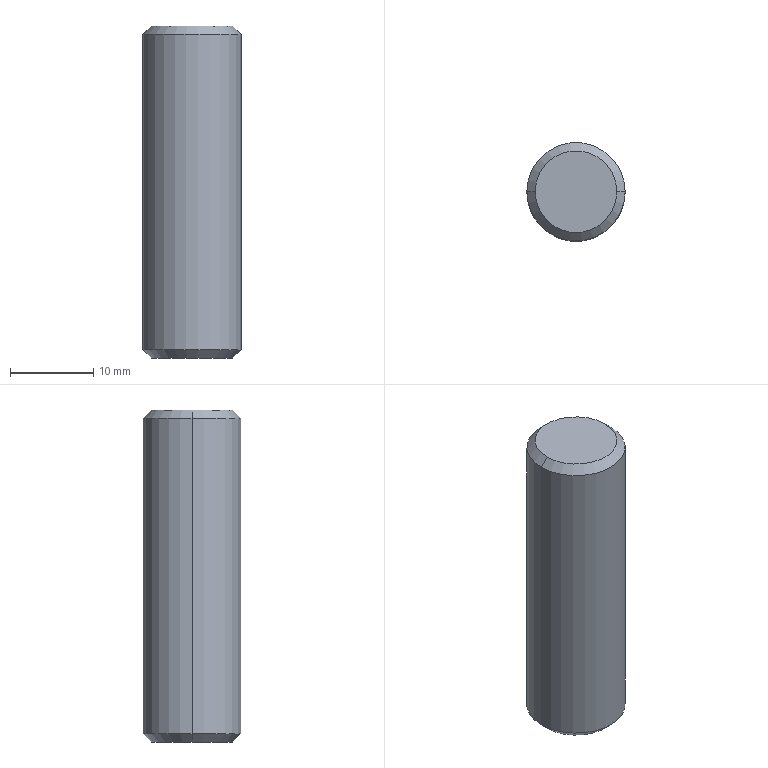Part | SolidWorks | features Chamfer 1, Extrusion 1 | 1 solid | 8 faces | box 11.85 x 11.85 x 40 mm | volume 4376 mm3 | cone 4 | cylinder 2 | plane 2 | commonest cylinder face diameters 11.85 x2
STEP:
#1=CARTESIAN_POINT('',(-4.925,0.,0.));
#2=VERTEX_POINT('',#1);
#3=CARTESIAN_POINT('',(4.925,0.,0.));
#4=VERTEX_POINT('',#3);
#5=CARTESIAN_POINT('',(0.,0.,0.));
#6=DIRECTION('',(0.,0.,-1.));
#7=DIRECTION('',(1.,0.,0.));
#8=AXIS2_PLACEMENT_3D('',#5,#6,#7);
#9=CIRCLE('',#8,4.925);
#10=EDGE_CURVE('',#2,#4,#9,.T.);
#11=ORIENTED_EDGE('',*,*,#10,.F.);
#12=CARTESIAN_POINT('',(-5.925,0.,1.));
#13=VERTEX_POINT('',#12);
#14=CARTESIAN_POINT('',(-5.925,0.,1.));
#15=DIRECTION('',(-0.7071,0.,0.7071));
#16=VECTOR('',#15,1000.);
#17=LINE('',#14,#16);
#18=EDGE_CURVE('',#2,#13,#17,.T.);
#19=ORIENTED_EDGE('',*,*,#18,.T.);
#20=CARTESIAN_POINT('',(5.925,0.,1.));
#21=VERTEX_POINT('',#20);
#22=CARTESIAN_POINT('',(0.,0.,1.));
#23=DIRECTION('',(0.,0.,1.));
#24=DIRECTION('',(1.,0.,0.));
#25=AXIS2_PLACEMENT_3D('',#22,#23,#24);
#26=CIRCLE('',#25,5.925);
#27=EDGE_CURVE('',#21,#13,#26,.T.);
#28=ORIENTED_EDGE('',*,*,#27,.F.);
#29=CARTESIAN_POINT('',(5.925,0.,1.));
#30=DIRECTION('',(0.7071,0.,0.7071));
#31=VECTOR('',#30,1000.);
#32=LINE('',#29,#31);
#33=EDGE_CURVE('',#4,#21,#32,.T.);
#34=ORIENTED_EDGE('',*,*,#33,.F.);
#35=EDGE_LOOP('',(#11,#19,#28,#34));
#36=FACE_OUTER_BOUND('',#35,.T.);
#37=CARTESIAN_POINT('',(0.,0.,1.));
#38=DIRECTION('',(0.,0.,1.));
#39=DIRECTION('',(1.,0.,0.));
#40=AXIS2_PLACEMENT_3D('',#37,#38,#39);
#41=CONICAL_SURFACE('',#40,5.925,0.7854);
#42=ADVANCED_FACE('',(#36),#41,.T.);
#43=CARTESIAN_POINT('',(4.925,0.,40.));
#44=VERTEX_POINT('',#43);
#45=CARTESIAN_POINT('',(-4.925,0.,40.));
#46=VERTEX_POINT('',#45);
#47=CARTESIAN_POINT('',(0.,0.,40.));
#48=DIRECTION('',(0.,0.,1.));
#49=DIRECTION('',(1.,0.,0.));
#50=AXIS2_PLACEMENT_3D('',#47,#48,#49);
#51=CIRCLE('',#50,4.925);
#52=EDGE_CURVE('',#44,#46,#51,.T.);
#53=ORIENTED_EDGE('',*,*,#52,.F.);
#54=CARTESIAN_POINT('',(5.925,0.,39.));
#55=VERTEX_POINT('',#54);
#56=CARTESIAN_POINT('',(4.925,0.,40.));
#57=DIRECTION('',(0.7071,0.,-0.7071));
#58=VECTOR('',#57,1000.);
#59=LINE('',#56,#58);
#60=EDGE_CURVE('',#44,#55,#59,.T.);
#61=ORIENTED_EDGE('',*,*,#60,.T.);
#62=CARTESIAN_POINT('',(-5.925,0.,39.));
#63=VERTEX_POINT('',#62);
#64=CARTESIAN_POINT('',(0.,0.,39.));
#65=DIRECTION('',(0.,0.,-1.));
#66=DIRECTION('',(1.,0.,0.));
#67=AXIS2_PLACEMENT_3D('',#64,#65,#66);
#68=CIRCLE('',#67,5.925);
#69=EDGE_CURVE('',#63,#55,#68,.T.);
#70=ORIENTED_EDGE('',*,*,#69,.F.);
#71=CARTESIAN_POINT('',(-4.925,0.,40.));
#72=DIRECTION('',(-0.7071,0.,-0.7071));
#73=VECTOR('',#72,1000.);
#74=LINE('',#71,#73);
#75=EDGE_CURVE('',#46,#63,#74,.T.);
#76=ORIENTED_EDGE('',*,*,#75,.F.);
#77=EDGE_LOOP('',(#53,#61,#70,#76));
#78=FACE_OUTER_BOUND('',#77,.T.);
#79=CARTESIAN_POINT('',(0.,0.,40.));
#80=DIRECTION('',(0.,0.,-1.));
#81=DIRECTION('',(-1.,0.,0.));
#82=AXIS2_PLACEMENT_3D('',#79,#80,#81);
#83=CONICAL_SURFACE('',#82,4.925,0.7854);
#84=ADVANCED_FACE('',(#78),#83,.T.);
#85=ORIENTED_EDGE('',*,*,#69,.T.);
#86=CARTESIAN_POINT('',(5.925,0.,40.));
#87=DIRECTION('',(0.,0.,-1.));
#88=VECTOR('',#87,1000.);
#89=LINE('',#86,#88);
#90=EDGE_CURVE('',#55,#21,#89,.T.);
#91=ORIENTED_EDGE('',*,*,#90,.T.);
#92=ORIENTED_EDGE('',*,*,#27,.T.);
#93=CARTESIAN_POINT('',(-5.925,0.,40.));
#94=DIRECTION('',(0.,0.,-1.));
#95=VECTOR('',#94,1000.);
#96=LINE('',#93,#95);
#97=EDGE_CURVE('',#63,#13,#96,.T.);
#98=ORIENTED_EDGE('',*,*,#97,.F.);
#99=EDGE_LOOP('',(#85,#91,#92,#98));
#100=FACE_OUTER_BOUND('',#99,.T.);
#101=CARTESIAN_POINT('',(0.,0.,40.));
#102=DIRECTION('',(0.,0.,-1.));
#103=DIRECTION('',(-1.,0.,0.));
#104=AXIS2_PLACEMENT_3D('',#101,#102,#103);
#105=CYLINDRICAL_SURFACE('',#104,5.925);
#106=ADVANCED_FACE('',(#100),#105,.T.);
#107=ORIENTED_EDGE('',*,*,#90,.F.);
#108=CARTESIAN_POINT('',(0.,0.,39.));
#109=DIRECTION('',(0.,0.,-1.));
#110=DIRECTION('',(1.,0.,0.));
#111=AXIS2_PLACEMENT_3D('',#108,#109,#110);
#112=CIRCLE('',#111,5.925);
#113=EDGE_CURVE('',#55,#63,#112,.T.);
#114=ORIENTED_EDGE('',*,*,#113,.T.);
#115=ORIENTED_EDGE('',*,*,#97,.T.);
#116=CARTESIAN_POINT('',(0.,0.,1.));
#117=DIRECTION('',(0.,0.,1.));
#118=DIRECTION('',(1.,0.,0.));
#119=AXIS2_PLACEMENT_3D('',#116,#117,#118);
#120=CIRCLE('',#119,5.925);
#121=EDGE_CURVE('',#13,#21,#120,.T.);
#122=ORIENTED_EDGE('',*,*,#121,.T.);
#123=EDGE_LOOP('',(#107,#114,#115,#122));
#124=FACE_OUTER_BOUND('',#123,.T.);
#125=CARTESIAN_POINT('',(0.,0.,40.));
#126=DIRECTION('',(0.,0.,-1.));
#127=DIRECTION('',(-1.,0.,0.));
#128=AXIS2_PLACEMENT_3D('',#125,#126,#127);
#129=CYLINDRICAL_SURFACE('',#128,5.925);
#130=ADVANCED_FACE('',(#124),#129,.T.);
#131=CARTESIAN_POINT('',(0.,0.,40.));
#132=DIRECTION('',(0.,0.,1.));
#133=DIRECTION('',(1.,0.,0.));
#134=AXIS2_PLACEMENT_3D('',#131,#132,#133);
#135=CIRCLE('',#134,4.925);
#136=EDGE_CURVE('',#46,#44,#135,.T.);
#137=ORIENTED_EDGE('',*,*,#136,.T.);
#138=ORIENTED_EDGE('',*,*,#52,.T.);
#139=EDGE_LOOP('',(#137,#138));
#140=FACE_OUTER_BOUND('',#139,.T.);
#141=CARTESIAN_POINT('',(0.,0.,40.));
#142=DIRECTION('',(0.,0.,1.));
#143=DIRECTION('',(1.,0.,0.));
#144=AXIS2_PLACEMENT_3D('',#141,#142,#143);
#145=PLANE('',#144);
#146=ADVANCED_FACE('',(#140),#145,.T.);
#147=CARTESIAN_POINT('',(0.,0.,0.));
#148=DIRECTION('',(0.,0.,-1.));
#149=DIRECTION('',(1.,0.,0.));
#150=AXIS2_PLACEMENT_3D('',#147,#148,#149);
#151=CIRCLE('',#150,4.925);
#152=EDGE_CURVE('',#4,#2,#151,.T.);
#153=ORIENTED_EDGE('',*,*,#152,.T.);
#154=ORIENTED_EDGE('',*,*,#10,.T.);
#155=EDGE_LOOP('',(#153,#154));
#156=FACE_OUTER_BOUND('',#155,.T.);
#157=CARTESIAN_POINT('',(0.,0.,0.));
#158=DIRECTION('',(0.,0.,1.));
#159=DIRECTION('',(1.,0.,0.));
#160=AXIS2_PLACEMENT_3D('',#157,#158,#159);
#161=PLANE('',#160);
#162=ADVANCED_FACE('',(#156),#161,.F.);
#163=ORIENTED_EDGE('',*,*,#60,.F.);
#164=ORIENTED_EDGE('',*,*,#136,.F.);
#165=ORIENTED_EDGE('',*,*,#75,.T.);
#166=ORIENTED_EDGE('',*,*,#113,.F.);
#167=EDGE_LOOP('',(#163,#164,#165,#166));
#168=FACE_OUTER_BOUND('',#167,.T.);
#169=CARTESIAN_POINT('',(0.,0.,40.));
#170=DIRECTION('',(0.,0.,-1.));
#171=DIRECTION('',(-1.,0.,0.));
#172=AXIS2_PLACEMENT_3D('',#169,#170,#171);
#173=CONICAL_SURFACE('',#172,4.925,0.7854);
#174=ADVANCED_FACE('',(#168),#173,.T.);
#175=ORIENTED_EDGE('',*,*,#18,.F.);
#176=ORIENTED_EDGE('',*,*,#152,.F.);
#177=ORIENTED_EDGE('',*,*,#33,.T.);
#178=ORIENTED_EDGE('',*,*,#121,.F.);
#179=EDGE_LOOP('',(#175,#176,#177,#178));
#180=FACE_OUTER_BOUND('',#179,.T.);
#181=CARTESIAN_POINT('',(0.,0.,1.));
#182=DIRECTION('',(0.,0.,1.));
#183=DIRECTION('',(1.,0.,0.));
#184=AXIS2_PLACEMENT_3D('',#181,#182,#183);
#185=CONICAL_SURFACE('',#184,5.925,0.7854);
#186=ADVANCED_FACE('',(#180),#185,.T.);
#187=CLOSED_SHELL('',(#42,#84,#106,#130,#146,#162,#174,#186));
#188=MANIFOLD_SOLID_BREP('',#187);
#189=CARTESIAN_POINT('',(0.,0.,0.));
#190=DIRECTION('',(0.,0.,1.));
#191=DIRECTION('',(1.,0.,0.));
#192=AXIS2_PLACEMENT_3D('',#189,#190,#191);
#193=(LENGTH_UNIT()NAMED_UNIT(*)SI_UNIT(.MILLI.,.METRE.));
#194=UNCERTAINTY_MEASURE_WITH_UNIT(LENGTH_MEASURE(0.00001),#193,'','');
#195=(NAMED_UNIT(*)PLANE_ANGLE_UNIT()SI_UNIT($,.RADIAN.));
#196=(NAMED_UNIT(*)SI_UNIT($,.STERADIAN.)SOLID_ANGLE_UNIT());
#197=(GEOMETRIC_REPRESENTATION_CONTEXT(3)GLOBAL_UNCERTAINTY_ASSIGNED_CONTEXT((#194))GLOBAL_UNIT_ASSIGNED_CONTEXT((#193,#195,#196))REPRESENTATION_CONTEXT('',''));
#198=ADVANCED_BREP_SHAPE_REPRESENTATION('',(#188,#192),#197);